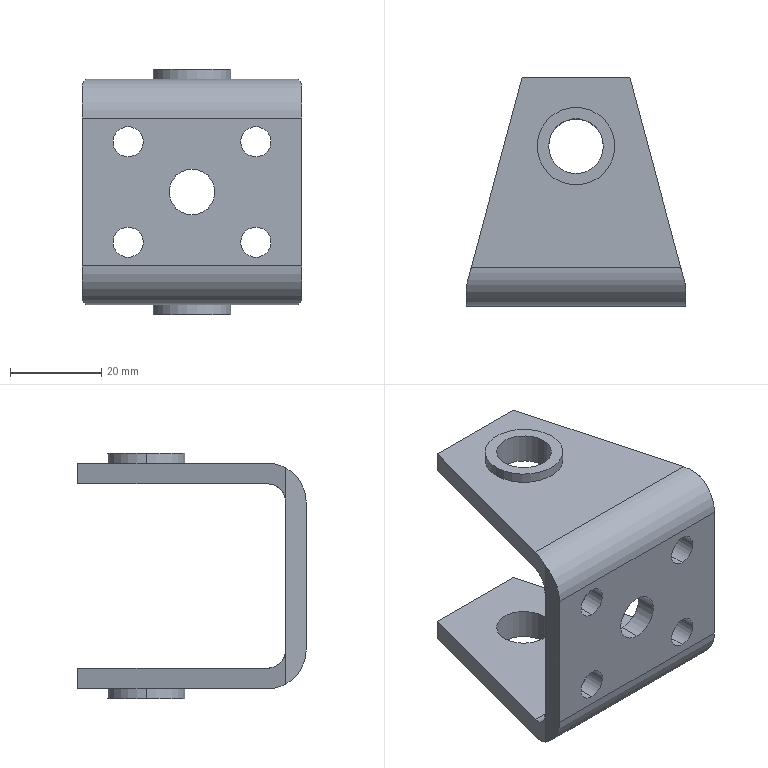Part | SolidWorks | features BaseBody 1 | 1 solid | 38 faces | box 48 x 50 x 53.8 mm | volume 22684 mm3 | cylinder 22 | plane 16 | commonest cylinder face diameters 6.6 x8 17 x6 12 x4 8 x2 10 x2
STEP:
#1=CARTESIAN_POINT('',(-8.5,0.,-24.7));
#2=VERTEX_POINT('',#1);
#3=CARTESIAN_POINT('',(8.5,0.,-24.7));
#4=VERTEX_POINT('',#3);
#5=CARTESIAN_POINT('',(0.,0.,-24.7));
#6=DIRECTION('',(0.,0.,-1.));
#7=DIRECTION('',(1.,0.,0.));
#8=AXIS2_PLACEMENT_3D('',#5,#6,#7);
#9=CIRCLE('',#8,8.5);
#10=EDGE_CURVE('',#2,#4,#9,.T.);
#11=ORIENTED_EDGE('',*,*,#10,.T.);
#12=CARTESIAN_POINT('',(8.5,0.,-26.9));
#13=VERTEX_POINT('',#12);
#14=CARTESIAN_POINT('',(8.5,0.,-26.9));
#15=DIRECTION('',(0.,0.,-1.));
#16=VECTOR('',#15,1000.);
#17=LINE('',#14,#16);
#18=EDGE_CURVE('',#4,#13,#17,.T.);
#19=ORIENTED_EDGE('',*,*,#18,.T.);
#20=CARTESIAN_POINT('',(-8.5,0.,-26.9));
#21=VERTEX_POINT('',#20);
#22=CARTESIAN_POINT('',(0.,0.,-26.9));
#23=DIRECTION('',(0.,0.,-1.));
#24=DIRECTION('',(-1.,0.,0.));
#25=AXIS2_PLACEMENT_3D('',#22,#23,#24);
#26=CIRCLE('',#25,8.5);
#27=EDGE_CURVE('',#21,#13,#26,.T.);
#28=ORIENTED_EDGE('',*,*,#27,.F.);
#29=CARTESIAN_POINT('',(-8.5,0.,-26.9));
#30=DIRECTION('',(0.,0.,-1.));
#31=VECTOR('',#30,1000.);
#32=LINE('',#29,#31);
#33=EDGE_CURVE('',#2,#21,#32,.T.);
#34=ORIENTED_EDGE('',*,*,#33,.F.);
#35=EDGE_LOOP('',(#11,#19,#28,#34));
#36=FACE_OUTER_BOUND('',#35,.T.);
#37=CARTESIAN_POINT('',(0.,0.,-26.9));
#38=DIRECTION('',(0.,0.,-1.));
#39=DIRECTION('',(-1.,0.,0.));
#40=AXIS2_PLACEMENT_3D('',#37,#38,#39);
#41=CYLINDRICAL_SURFACE('',#40,8.5);
#42=ADVANCED_FACE('',(#36),#41,.T.);
#43=CARTESIAN_POINT('',(-6.,0.,-20.2));
#44=VERTEX_POINT('',#43);
#45=CARTESIAN_POINT('',(6.,0.,-20.2));
#46=VERTEX_POINT('',#45);
#47=CARTESIAN_POINT('',(0.,0.,-20.2));
#48=DIRECTION('',(0.,0.,1.));
#49=DIRECTION('',(-1.,0.,0.));
#50=AXIS2_PLACEMENT_3D('',#47,#48,#49);
#51=CIRCLE('',#50,6.);
#52=EDGE_CURVE('',#44,#46,#51,.T.);
#53=ORIENTED_EDGE('',*,*,#52,.T.);
#54=CARTESIAN_POINT('',(6.,0.,-26.9));
#55=VERTEX_POINT('',#54);
#56=CARTESIAN_POINT('',(6.,0.,53.8));
#57=DIRECTION('',(0.,0.,-1.));
#58=VECTOR('',#57,1000.);
#59=LINE('',#56,#58);
#60=EDGE_CURVE('',#46,#55,#59,.T.);
#61=ORIENTED_EDGE('',*,*,#60,.T.);
#62=CARTESIAN_POINT('',(-6.,0.,-26.9));
#63=VERTEX_POINT('',#62);
#64=CARTESIAN_POINT('',(0.,0.,-26.9));
#65=DIRECTION('',(0.,0.,-1.));
#66=DIRECTION('',(1.,0.,0.));
#67=AXIS2_PLACEMENT_3D('',#64,#65,#66);
#68=CIRCLE('',#67,6.);
#69=EDGE_CURVE('',#55,#63,#68,.T.);
#70=ORIENTED_EDGE('',*,*,#69,.T.);
#71=CARTESIAN_POINT('',(-6.,0.,53.8));
#72=DIRECTION('',(0.,0.,-1.));
#73=VECTOR('',#72,1000.);
#74=LINE('',#71,#73);
#75=EDGE_CURVE('',#44,#63,#74,.T.);
#76=ORIENTED_EDGE('',*,*,#75,.F.);
#77=EDGE_LOOP('',(#53,#61,#70,#76));
#78=FACE_OUTER_BOUND('',#77,.T.);
#79=CARTESIAN_POINT('',(0.,0.,53.8));
#80=DIRECTION('',(0.,0.,-1.));
#81=DIRECTION('',(-1.,0.,0.));
#82=AXIS2_PLACEMENT_3D('',#79,#80,#81);
#83=CYLINDRICAL_SURFACE('',#82,6.);
#84=ADVANCED_FACE('',(#78),#83,.F.);
#85=CARTESIAN_POINT('',(0.,-35.,-5.));
#86=VERTEX_POINT('',#85);
#87=CARTESIAN_POINT('',(0.,-35.,5.));
#88=VERTEX_POINT('',#87);
#89=CARTESIAN_POINT('',(0.,-35.,0.));
#90=DIRECTION('',(0.,1.,0.));
#91=DIRECTION('',(0.,0.,1.));
#92=AXIS2_PLACEMENT_3D('',#89,#90,#91);
#93=CIRCLE('',#92,5.);
#94=EDGE_CURVE('',#86,#88,#93,.T.);
#95=ORIENTED_EDGE('',*,*,#94,.F.);
#96=CARTESIAN_POINT('',(0.,-30.5,-5.));
#97=VERTEX_POINT('',#96);
#98=CARTESIAN_POINT('',(0.,-50.,-5.));
#99=DIRECTION('',(0.,1.,0.));
#100=VECTOR('',#99,1000.);
#101=LINE('',#98,#100);
#102=EDGE_CURVE('',#86,#97,#101,.T.);
#103=ORIENTED_EDGE('',*,*,#102,.T.);
#104=CARTESIAN_POINT('',(0.,-30.5,5.));
#105=VERTEX_POINT('',#104);
#106=CARTESIAN_POINT('',(0.,-30.5,0.));
#107=DIRECTION('',(0.,-1.,0.));
#108=DIRECTION('',(0.,0.,-1.));
#109=AXIS2_PLACEMENT_3D('',#106,#107,#108);
#110=CIRCLE('',#109,5.);
#111=EDGE_CURVE('',#105,#97,#110,.T.);
#112=ORIENTED_EDGE('',*,*,#111,.F.);
#113=CARTESIAN_POINT('',(0.,-50.,5.));
#114=DIRECTION('',(0.,1.,0.));
#115=VECTOR('',#114,1000.);
#116=LINE('',#113,#115);
#117=EDGE_CURVE('',#88,#105,#116,.T.);
#118=ORIENTED_EDGE('',*,*,#117,.F.);
#119=EDGE_LOOP('',(#95,#103,#112,#118));
#120=FACE_OUTER_BOUND('',#119,.T.);
#121=CARTESIAN_POINT('',(0.,-50.,0.));
#122=DIRECTION('',(0.,1.,0.));
#123=DIRECTION('',(0.,0.,1.));
#124=AXIS2_PLACEMENT_3D('',#121,#122,#123);
#125=CYLINDRICAL_SURFACE('',#124,5.);
#126=ADVANCED_FACE('',(#120),#125,.F.);
#127=CARTESIAN_POINT('',(14.,-35.,-14.3));
#128=VERTEX_POINT('',#127);
#129=CARTESIAN_POINT('',(14.,-35.,-7.7));
#130=VERTEX_POINT('',#129);
#131=CARTESIAN_POINT('',(14.,-35.,-11.));
#132=DIRECTION('',(0.,1.,0.));
#133=DIRECTION('',(0.,0.,1.));
#134=AXIS2_PLACEMENT_3D('',#131,#132,#133);
#135=CIRCLE('',#134,3.3);
#136=EDGE_CURVE('',#128,#130,#135,.T.);
#137=ORIENTED_EDGE('',*,*,#136,.F.);
#138=CARTESIAN_POINT('',(14.,-30.5,-14.3));
#139=VERTEX_POINT('',#138);
#140=CARTESIAN_POINT('',(14.,-50.,-14.3));
#141=DIRECTION('',(0.,1.,0.));
#142=VECTOR('',#141,1000.);
#143=LINE('',#140,#142);
#144=EDGE_CURVE('',#128,#139,#143,.T.);
#145=ORIENTED_EDGE('',*,*,#144,.T.);
#146=CARTESIAN_POINT('',(14.,-30.5,-7.7));
#147=VERTEX_POINT('',#146);
#148=CARTESIAN_POINT('',(14.,-30.5,-11.));
#149=DIRECTION('',(0.,-1.,0.));
#150=DIRECTION('',(0.,0.,-1.));
#151=AXIS2_PLACEMENT_3D('',#148,#149,#150);
#152=CIRCLE('',#151,3.3);
#153=EDGE_CURVE('',#147,#139,#152,.T.);
#154=ORIENTED_EDGE('',*,*,#153,.F.);
#155=CARTESIAN_POINT('',(14.,-50.,-7.7));
#156=DIRECTION('',(0.,1.,0.));
#157=VECTOR('',#156,1000.);
#158=LINE('',#155,#157);
#159=EDGE_CURVE('',#130,#147,#158,.T.);
#160=ORIENTED_EDGE('',*,*,#159,.F.);
#161=EDGE_LOOP('',(#137,#145,#154,#160));
#162=FACE_OUTER_BOUND('',#161,.T.);
#163=CARTESIAN_POINT('',(14.,-50.,-11.));
#164=DIRECTION('',(0.,1.,0.));
#165=DIRECTION('',(0.,0.,1.));
#166=AXIS2_PLACEMENT_3D('',#163,#164,#165);
#167=CYLINDRICAL_SURFACE('',#166,3.3);
#168=ADVANCED_FACE('',(#162),#167,.F.);
#169=CARTESIAN_POINT('',(-14.,-35.,-14.3));
#170=VERTEX_POINT('',#169);
#171=CARTESIAN_POINT('',(-14.,-35.,-7.7));
#172=VERTEX_POINT('',#171);
#173=CARTESIAN_POINT('',(-14.,-35.,-11.));
#174=DIRECTION('',(0.,1.,0.));
#175=DIRECTION('',(0.,0.,1.));
#176=AXIS2_PLACEMENT_3D('',#173,#174,#175);
#177=CIRCLE('',#176,3.3);
#178=EDGE_CURVE('',#170,#172,#177,.T.);
#179=ORIENTED_EDGE('',*,*,#178,.F.);
#180=CARTESIAN_POINT('',(-14.,-30.5,-14.3));
#181=VERTEX_POINT('',#180);
#182=CARTESIAN_POINT('',(-14.,-50.,-14.3));
#183=DIRECTION('',(0.,1.,0.));
#184=VECTOR('',#183,1000.);
#185=LINE('',#182,#184);
#186=EDGE_CURVE('',#170,#181,#185,.T.);
#187=ORIENTED_EDGE('',*,*,#186,.T.);
#188=CARTESIAN_POINT('',(-14.,-30.5,-7.7));
#189=VERTEX_POINT('',#188);
#190=CARTESIAN_POINT('',(-14.,-30.5,-11.));
#191=DIRECTION('',(0.,-1.,0.));
#192=DIRECTION('',(0.,0.,-1.));
#193=AXIS2_PLACEMENT_3D('',#190,#191,#192);
#194=CIRCLE('',#193,3.3);
#195=EDGE_CURVE('',#189,#181,#194,.T.);
#196=ORIENTED_EDGE('',*,*,#195,.F.);
#197=CARTESIAN_POINT('',(-14.,-50.,-7.7));
#198=DIRECTION('',(0.,1.,0.));
#199=VECTOR('',#198,1000.);
#200=LINE('',#197,#199);
#201=EDGE_CURVE('',#172,#189,#200,.T.);
#202=ORIENTED_EDGE('',*,*,#201,.F.);
#203=EDGE_LOOP('',(#179,#187,#196,#202));
#204=FACE_OUTER_BOUND('',#203,.T.);
#205=CARTESIAN_POINT('',(-14.,-50.,-11.));
#206=DIRECTION('',(0.,1.,0.));
#207=DIRECTION('',(0.,0.,1.));
#208=AXIS2_PLACEMENT_3D('',#205,#206,#207);
#209=CYLINDRICAL_SURFACE('',#208,3.3);
#210=ADVANCED_FACE('',(#204),#209,.F.);
#211=CARTESIAN_POINT('',(-14.,-35.,7.7));
#212=VERTEX_POINT('',#211);
#213=CARTESIAN_POINT('',(-14.,-35.,14.3));
#214=VERTEX_POINT('',#213);
#215=CARTESIAN_POINT('',(-14.,-35.,11.));
#216=DIRECTION('',(0.,1.,0.));
#217=DIRECTION('',(0.,0.,1.));
#218=AXIS2_PLACEMENT_3D('',#215,#216,#217);
#219=CIRCLE('',#218,3.3);
#220=EDGE_CURVE('',#212,#214,#219,.T.);
#221=ORIENTED_EDGE('',*,*,#220,.F.);
#222=CARTESIAN_POINT('',(-14.,-30.5,7.7));
#223=VERTEX_POINT('',#222);
#224=CARTESIAN_POINT('',(-14.,-50.,7.7));
#225=DIRECTION('',(0.,1.,0.));
#226=VECTOR('',#225,1000.);
#227=LINE('',#224,#226);
#228=EDGE_CURVE('',#212,#223,#227,.T.);
#229=ORIENTED_EDGE('',*,*,#228,.T.);
#230=CARTESIAN_POINT('',(-14.,-30.5,14.3));
#231=VERTEX_POINT('',#230);
#232=CARTESIAN_POINT('',(-14.,-30.5,11.));
#233=DIRECTION('',(0.,-1.,0.));
#234=DIRECTION('',(0.,0.,-1.));
#235=AXIS2_PLACEMENT_3D('',#232,#233,#234);
#236=CIRCLE('',#235,3.3);
#237=EDGE_CURVE('',#231,#223,#236,.T.);
#238=ORIENTED_EDGE('',*,*,#237,.F.);
#239=CARTESIAN_POINT('',(-14.,-50.,14.3));
#240=DIRECTION('',(0.,1.,0.));
#241=VECTOR('',#240,1000.);
#242=LINE('',#239,#241);
#243=EDGE_CURVE('',#214,#231,#242,.T.);
#244=ORIENTED_EDGE('',*,*,#243,.F.);
#245=EDGE_LOOP('',(#221,#229,#238,#244));
#246=FACE_OUTER_BOUND('',#245,.T.);
#247=CARTESIAN_POINT('',(-14.,-50.,11.));
#248=DIRECTION('',(0.,1.,0.));
#249=DIRECTION('',(0.,0.,1.));
#250=AXIS2_PLACEMENT_3D('',#247,#248,#249);
#251=CYLINDRICAL_SURFACE('',#250,3.3);
#252=ADVANCED_FACE('',(#246),#251,.F.);
#253=CARTESIAN_POINT('',(14.,-35.,7.7));
#254=VERTEX_POINT('',#253);
#255=CARTESIAN_POINT('',(14.,-35.,14.3));
#256=VERTEX_POINT('',#255);
#257=CARTESIAN_POINT('',(14.,-35.,11.));
#258=DIRECTION('',(0.,1.,0.));
#259=DIRECTION('',(0.,0.,1.));
#260=AXIS2_PLACEMENT_3D('',#257,#258,#259);
#261=CIRCLE('',#260,3.3);
#262=EDGE_CURVE('',#254,#256,#261,.T.);
#263=ORIENTED_EDGE('',*,*,#262,.F.);
#264=CARTESIAN_POINT('',(14.,-30.5,7.7));
#265=VERTEX_POINT('',#264);
#266=CARTESIAN_POINT('',(14.,-50.,7.7));
#267=DIRECTION('',(0.,1.,0.));
#268=VECTOR('',#267,1000.);
#269=LINE('',#266,#268);
#270=EDGE_CURVE('',#254,#265,#269,.T.);
#271=ORIENTED_EDGE('',*,*,#270,.T.);
#272=CARTESIAN_POINT('',(14.,-30.5,14.3));
#273=VERTEX_POINT('',#272);
#274=CARTESIAN_POINT('',(14.,-30.5,11.));
#275=DIRECTION('',(0.,-1.,0.));
#276=DIRECTION('',(0.,0.,-1.));
#277=AXIS2_PLACEMENT_3D('',#274,#275,#276);
#278=CIRCLE('',#277,3.3);
#279=EDGE_CURVE('',#273,#265,#278,.T.);
#280=ORIENTED_EDGE('',*,*,#279,.F.);
#281=CARTESIAN_POINT('',(14.,-50.,14.3));
#282=DIRECTION('',(0.,1.,0.));
#283=VECTOR('',#282,1000.);
#284=LINE('',#281,#283);
#285=EDGE_CURVE('',#256,#273,#284,.T.);
#286=ORIENTED_EDGE('',*,*,#285,.F.);
#287=EDGE_LOOP('',(#263,#271,#280,#286));
#288=FACE_OUTER_BOUND('',#287,.T.);
#289=CARTESIAN_POINT('',(14.,-50.,11.));
#290=DIRECTION('',(0.,1.,0.));
#291=DIRECTION('',(0.,0.,1.));
#292=AXIS2_PLACEMENT_3D('',#289,#290,#291);
#293=CYLINDRICAL_SURFACE('',#292,3.3);
#294=ADVANCED_FACE('',(#288),#293,.F.);
#295=CARTESIAN_POINT('',(-8.5,0.,26.9));
#296=VERTEX_POINT('',#295);
#297=CARTESIAN_POINT('',(8.5,0.,26.9));
#298=VERTEX_POINT('',#297);
#299=CARTESIAN_POINT('',(0.,0.,26.9));
#300=DIRECTION('',(0.,0.,-1.));
#301=DIRECTION('',(-1.,0.,0.));
#302=AXIS2_PLACEMENT_3D('',#299,#300,#301);
#303=CIRCLE('',#302,8.5);
#304=EDGE_CURVE('',#296,#298,#303,.T.);
#305=ORIENTED_EDGE('',*,*,#304,.T.);
#306=CARTESIAN_POINT('',(8.5,0.,24.7));
#307=VERTEX_POINT('',#306);
#308=CARTESIAN_POINT('',(8.5,0.,-26.9));
#309=DIRECTION('',(0.,0.,-1.));
#310=VECTOR('',#309,1000.);
#311=LINE('',#308,#310);
#312=EDGE_CURVE('',#298,#307,#311,.T.);
#313=ORIENTED_EDGE('',*,*,#312,.T.);
#314=CARTESIAN_POINT('',(-8.5,0.,24.7));
#315=VERTEX_POINT('',#314);
#316=CARTESIAN_POINT('',(0.,0.,24.7));
#317=DIRECTION('',(0.,0.,1.));
#318=DIRECTION('',(-1.,0.,0.));
#319=AXIS2_PLACEMENT_3D('',#316,#317,#318);
#320=CIRCLE('',#319,8.5);
#321=EDGE_CURVE('',#307,#315,#320,.T.);
#322=ORIENTED_EDGE('',*,*,#321,.T.);
#323=CARTESIAN_POINT('',(-8.5,0.,-26.9));
#324=DIRECTION('',(0.,0.,-1.));
#325=VECTOR('',#324,1000.);
#326=LINE('',#323,#325);
#327=EDGE_CURVE('',#296,#315,#326,.T.);
#328=ORIENTED_EDGE('',*,*,#327,.F.);
#329=EDGE_LOOP('',(#305,#313,#322,#328));
#330=FACE_OUTER_BOUND('',#329,.T.);
#331=CARTESIAN_POINT('',(0.,0.,-26.9));
#332=DIRECTION('',(0.,0.,-1.));
#333=DIRECTION('',(-1.,0.,0.));
#334=AXIS2_PLACEMENT_3D('',#331,#332,#333);
#335=CYLINDRICAL_SURFACE('',#334,8.5);
#336=ADVANCED_FACE('',(#330),#335,.T.);
#337=CARTESIAN_POINT('',(-6.,0.,26.9));
#338=VERTEX_POINT('',#337);
#339=CARTESIAN_POINT('',(6.,0.,26.9));
#340=VERTEX_POINT('',#339);
#341=CARTESIAN_POINT('',(0.,0.,26.9));
#342=DIRECTION('',(0.,0.,1.));
#343=DIRECTION('',(-1.,0.,0.));
#344=AXIS2_PLACEMENT_3D('',#341,#342,#343);
#345=CIRCLE('',#344,6.);
#346=EDGE_CURVE('',#338,#340,#345,.T.);
#347=ORIENTED_EDGE('',*,*,#346,.T.);
#348=CARTESIAN_POINT('',(6.,0.,20.2));
#349=VERTEX_POINT('',#348);
#350=CARTESIAN_POINT('',(6.,0.,53.8));
#351=DIRECTION('',(0.,0.,-1.));
#352=VECTOR('',#351,1000.);
#353=LINE('',#350,#352);
#354=EDGE_CURVE('',#340,#349,#353,.T.);
#355=ORIENTED_EDGE('',*,*,#354,.T.);
#356=CARTESIAN_POINT('',(-6.,0.,20.2));
#357=VERTEX_POINT('',#356);
#358=CARTESIAN_POINT('',(0.,0.,20.2));
#359=DIRECTION('',(0.,0.,-1.));
#360=DIRECTION('',(1.,0.,0.));
#361=AXIS2_PLACEMENT_3D('',#358,#359,#360);
#362=CIRCLE('',#361,6.);
#363=EDGE_CURVE('',#349,#357,#362,.T.);
#364=ORIENTED_EDGE('',*,*,#363,.T.);
#365=CARTESIAN_POINT('',(-6.,0.,53.8));
#366=DIRECTION('',(0.,0.,-1.));
#367=VECTOR('',#366,1000.);
#368=LINE('',#365,#367);
#369=EDGE_CURVE('',#338,#357,#368,.T.);
#370=ORIENTED_EDGE('',*,*,#369,.F.);
#371=EDGE_LOOP('',(#347,#355,#364,#370));
#372=FACE_OUTER_BOUND('',#371,.T.);
#373=CARTESIAN_POINT('',(0.,0.,53.8));
#374=DIRECTION('',(0.,0.,-1.));
#375=DIRECTION('',(-1.,0.,0.));
#376=AXIS2_PLACEMENT_3D('',#373,#374,#375);
#377=CYLINDRICAL_SURFACE('',#376,6.);
#378=ADVANCED_FACE('',(#372),#377,.F.);
#379=CARTESIAN_POINT('',(11.8,15.,20.2));
#380=VERTEX_POINT('',#379);
#381=CARTESIAN_POINT('',(-11.8,15.,20.2));
#382=VERTEX_POINT('',#381);
#383=CARTESIAN_POINT('',(11.8,15.,20.2));
#384=DIRECTION('',(-1.,0.,0.));
#385=VECTOR('',#384,1000.);
#386=LINE('',#383,#385);
#387=EDGE_CURVE('',#380,#382,#386,.T.);
#388=ORIENTED_EDGE('',*,*,#387,.T.);
#389=CARTESIAN_POINT('',(-11.8,15.,24.7));
#390=VERTEX_POINT('',#389);
#391=CARTESIAN_POINT('',(-11.8,15.,24.7));
#392=DIRECTION('',(0.,0.,-1.));
#393=VECTOR('',#392,1000.);
#394=LINE('',#391,#393);
#395=EDGE_CURVE('',#390,#382,#394,.T.);
#396=ORIENTED_EDGE('',*,*,#395,.F.);
#397=CARTESIAN_POINT('',(11.8,15.,24.7));
#398=VERTEX_POINT('',#397);
#399=CARTESIAN_POINT('',(11.8,15.,24.7));
#400=DIRECTION('',(-1.,0.,0.));
#401=VECTOR('',#400,1000.);
#402=LINE('',#399,#401);
#403=EDGE_CURVE('',#398,#390,#402,.T.);
#404=ORIENTED_EDGE('',*,*,#403,.F.);
#405=CARTESIAN_POINT('',(11.8,15.,24.7));
#406=DIRECTION('',(0.,0.,-1.));
#407=VECTOR('',#406,1000.);
#408=LINE('',#405,#407);
#409=EDGE_CURVE('',#398,#380,#408,.T.);
#410=ORIENTED_EDGE('',*,*,#409,.T.);
#411=EDGE_LOOP('',(#388,#396,#404,#410));
#412=FACE_OUTER_BOUND('',#411,.T.);
#413=CARTESIAN_POINT('',(24.,15.,20.2));
#414=DIRECTION('',(0.,-1.,0.));
#415=DIRECTION('',(0.,0.,-1.));
#416=AXIS2_PLACEMENT_3D('',#413,#414,#415);
#417=PLANE('',#416);
#418=ADVANCED_FACE('',(#412),#417,.F.);
#419=CARTESIAN_POINT('',(0.,0.,20.2));
#420=DIRECTION('',(0.,0.,-1.));
#421=DIRECTION('',(1.,0.,0.));
#422=AXIS2_PLACEMENT_3D('',#419,#420,#421);
#423=CIRCLE('',#422,6.);
#424=EDGE_CURVE('',#357,#349,#423,.T.);
#425=ORIENTED_EDGE('',*,*,#424,.F.);
#426=ORIENTED_EDGE('',*,*,#363,.F.);
#427=EDGE_LOOP('',(#425,#426));
#428=FACE_BOUND('',#427,.T.);
#429=CARTESIAN_POINT('',(22.927,-26.5,20.2));
#430=VERTEX_POINT('',#429);
#431=CARTESIAN_POINT('',(-22.927,-26.5,20.2));
#432=VERTEX_POINT('',#431);
#433=CARTESIAN_POINT('',(22.927,-26.5,20.2));
#434=DIRECTION('',(-1.,0.,0.));
#435=VECTOR('',#434,1000.);
#436=LINE('',#433,#435);
#437=EDGE_CURVE('',#430,#432,#436,.T.);
#438=ORIENTED_EDGE('',*,*,#437,.T.);
#439=CARTESIAN_POINT('',(-22.927,-26.5,20.2));
#440=DIRECTION('',(0.259,0.9659,0.));
#441=VECTOR('',#440,1000.);
#442=LINE('',#439,#441);
#443=EDGE_CURVE('',#432,#382,#442,.T.);
#444=ORIENTED_EDGE('',*,*,#443,.T.);
#445=ORIENTED_EDGE('',*,*,#387,.F.);
#446=CARTESIAN_POINT('',(11.8,15.,20.2));
#447=DIRECTION('',(0.259,-0.9659,0.));
#448=VECTOR('',#447,1000.);
#449=LINE('',#446,#448);
#450=EDGE_CURVE('',#380,#430,#449,.T.);
#451=ORIENTED_EDGE('',*,*,#450,.T.);
#452=EDGE_LOOP('',(#438,#444,#445,#451));
#453=FACE_OUTER_BOUND('',#452,.T.);
#454=CARTESIAN_POINT('',(24.,-26.5,20.2));
#455=DIRECTION('',(0.,0.,1.));
#456=DIRECTION('',(1.,0.,0.));
#457=AXIS2_PLACEMENT_3D('',#454,#455,#456);
#458=PLANE('',#457);
#459=ADVANCED_FACE('',(#428,#453),#458,.F.);
#460=ORIENTED_EDGE('',*,*,#395,.T.);
#461=ORIENTED_EDGE('',*,*,#443,.F.);
#462=CARTESIAN_POINT('',(-24.,-30.5,16.2));
#463=VERTEX_POINT('',#462);
#464=CARTESIAN_POINT('',(-22.927,-26.5,20.2));
#465=CARTESIAN_POINT('',(-23.069,-27.029,20.2));
#466=CARTESIAN_POINT('',(-23.207,-27.542,20.098));
#467=CARTESIAN_POINT('',(-23.469,-28.519,19.693));
#468=CARTESIAN_POINT('',(-23.585,-28.954,19.403));
#469=CARTESIAN_POINT('',(-23.736,-29.515,18.842));
#470=CARTESIAN_POINT('',(-23.781,-29.682,18.639));
#471=CARTESIAN_POINT('',(-23.858,-29.971,18.206));
#472=CARTESIAN_POINT('',(-23.891,-30.094,17.976));
#473=CARTESIAN_POINT('',(-23.973,-30.398,17.241));
#474=CARTESIAN_POINT('',(-24.,-30.5,16.732));
#475=CARTESIAN_POINT('',(-24.,-30.5,16.2));
#476=B_SPLINE_CURVE_WITH_KNOTS('',3,(#464,#465,#466,#467,#468,#469,#470,#471,#472,#473,#474,#475),.UNSPECIFIED.,.F.,.F.,(4,2,2,2,2,4),(4.712,5.105,5.498,5.694,5.89,6.283),.UNSPECIFIED.);
#477=EDGE_CURVE('',#432,#463,#476,.T.);
#478=ORIENTED_EDGE('',*,*,#477,.T.);
#479=CARTESIAN_POINT('',(-24.,-30.5,23.7));
#480=VERTEX_POINT('',#479);
#481=CARTESIAN_POINT('',(-24.,-30.5,23.7));
#482=DIRECTION('',(0.,0.,-1.));
#483=VECTOR('',#482,1000.);
#484=LINE('',#481,#483);
#485=EDGE_CURVE('',#480,#463,#484,.T.);
#486=ORIENTED_EDGE('',*,*,#485,.F.);
#487=CARTESIAN_POINT('',(-22.927,-26.5,24.7));
#488=VERTEX_POINT('',#487);
#489=CARTESIAN_POINT('',(-22.927,-26.5,24.7));
#490=CARTESIAN_POINT('',(-23.113,-27.194,24.7));
#491=CARTESIAN_POINT('',(-23.3,-27.889,24.614));
#492=CARTESIAN_POINT('',(-23.661,-29.235,24.278));
#493=CARTESIAN_POINT('',(-23.835,-29.886,24.028));
#494=CARTESIAN_POINT('',(-24.,-30.5,23.7));
#495=B_SPLINE_CURVE_WITH_KNOTS('',3,(#489,#490,#491,#492,#493,#494),.UNSPECIFIED.,.F.,.F.,(4,2,4),(4.712,4.957,5.202),.UNSPECIFIED.);
#496=EDGE_CURVE('',#488,#480,#495,.T.);
#497=ORIENTED_EDGE('',*,*,#496,.F.);
#498=CARTESIAN_POINT('',(-11.8,15.,24.7));
#499=DIRECTION('',(-0.259,-0.9659,0.));
#500=VECTOR('',#499,1000.);
#501=LINE('',#498,#500);
#502=EDGE_CURVE('',#390,#488,#501,.T.);
#503=ORIENTED_EDGE('',*,*,#502,.F.);
#504=EDGE_LOOP('',(#460,#461,#478,#486,#497,#503));
#505=FACE_OUTER_BOUND('',#504,.T.);
#506=CARTESIAN_POINT('',(-11.8,15.,53.8));
#507=DIRECTION('',(0.9659,-0.259,0.));
#508=DIRECTION('',(0.259,0.9659,0.));
#509=AXIS2_PLACEMENT_3D('',#506,#507,#508);
#510=PLANE('',#509);
#511=ADVANCED_FACE('',(#505),#510,.F.);
#512=CARTESIAN_POINT('',(0.,0.,24.7));
#513=DIRECTION('',(0.,0.,1.));
#514=DIRECTION('',(-1.,0.,0.));
#515=AXIS2_PLACEMENT_3D('',#512,#513,#514);
#516=CIRCLE('',#515,8.5);
#517=EDGE_CURVE('',#315,#307,#516,.T.);
#518=ORIENTED_EDGE('',*,*,#517,.F.);
#519=ORIENTED_EDGE('',*,*,#321,.F.);
#520=EDGE_LOOP('',(#518,#519));
#521=FACE_BOUND('',#520,.T.);
#522=ORIENTED_EDGE('',*,*,#403,.T.);
#523=ORIENTED_EDGE('',*,*,#502,.T.);
#524=CARTESIAN_POINT('',(22.927,-26.5,24.7));
#525=VERTEX_POINT('',#524);
#526=CARTESIAN_POINT('',(22.927,-26.5,24.7));
#527=DIRECTION('',(-1.,0.,0.));
#528=VECTOR('',#527,1000.);
#529=LINE('',#526,#528);
#530=EDGE_CURVE('',#525,#488,#529,.T.);
#531=ORIENTED_EDGE('',*,*,#530,.F.);
#532=CARTESIAN_POINT('',(22.927,-26.5,24.7));
#533=DIRECTION('',(-0.259,0.9659,0.));
#534=VECTOR('',#533,1000.);
#535=LINE('',#532,#534);
#536=EDGE_CURVE('',#525,#398,#535,.T.);
#537=ORIENTED_EDGE('',*,*,#536,.T.);
#538=EDGE_LOOP('',(#522,#523,#531,#537));
#539=FACE_OUTER_BOUND('',#538,.T.);
#540=CARTESIAN_POINT('',(24.,15.,24.7));
#541=DIRECTION('',(0.,0.,-1.));
#542=DIRECTION('',(-1.,0.,0.));
#543=AXIS2_PLACEMENT_3D('',#540,#541,#542);
#544=PLANE('',#543);
#545=ADVANCED_FACE('',(#521,#539),#544,.F.);
#546=CARTESIAN_POINT('',(24.,-30.5,23.7));
#547=VERTEX_POINT('',#546);
#548=CARTESIAN_POINT('',(24.,-30.5,23.7));
#549=CARTESIAN_POINT('',(23.835,-29.886,24.028));
#550=CARTESIAN_POINT('',(23.661,-29.235,24.278));
#551=CARTESIAN_POINT('',(23.3,-27.889,24.614));
#552=CARTESIAN_POINT('',(23.113,-27.194,24.7));
#553=CARTESIAN_POINT('',(22.927,-26.5,24.7));
#554=B_SPLINE_CURVE_WITH_KNOTS('',3,(#548,#549,#550,#551,#552,#553),.UNSPECIFIED.,.F.,.F.,(4,2,4),(4.222,4.467,4.712),.UNSPECIFIED.);
#555=EDGE_CURVE('',#547,#525,#554,.T.);
#556=ORIENTED_EDGE('',*,*,#555,.F.);
#557=CARTESIAN_POINT('',(24.,-30.5,16.2));
#558=VERTEX_POINT('',#557);
#559=CARTESIAN_POINT('',(24.,-30.5,23.7));
#560=DIRECTION('',(0.,0.,-1.));
#561=VECTOR('',#560,1000.);
#562=LINE('',#559,#561);
#563=EDGE_CURVE('',#547,#558,#562,.T.);
#564=ORIENTED_EDGE('',*,*,#563,.T.);
#565=CARTESIAN_POINT('',(24.,-30.5,16.2));
#566=CARTESIAN_POINT('',(24.,-30.5,16.732));
#567=CARTESIAN_POINT('',(23.973,-30.398,17.241));
#568=CARTESIAN_POINT('',(23.891,-30.094,17.976));
#569=CARTESIAN_POINT('',(23.858,-29.971,18.206));
#570=CARTESIAN_POINT('',(23.781,-29.682,18.639));
#571=CARTESIAN_POINT('',(23.736,-29.515,18.842));
#572=CARTESIAN_POINT('',(23.585,-28.954,19.403));
#573=CARTESIAN_POINT('',(23.469,-28.519,19.693));
#574=CARTESIAN_POINT('',(23.207,-27.542,20.098));
#575=CARTESIAN_POINT('',(23.069,-27.029,20.2));
#576=CARTESIAN_POINT('',(22.927,-26.5,20.2));
#577=B_SPLINE_CURVE_WITH_KNOTS('',3,(#565,#566,#567,#568,#569,#570,#571,#572,#573,#574,#575,#576),.UNSPECIFIED.,.F.,.F.,(4,2,2,2,2,4),(3.142,3.534,3.731,3.927,4.32,4.712),.UNSPECIFIED.);
#578=EDGE_CURVE('',#558,#430,#577,.T.);
#579=ORIENTED_EDGE('',*,*,#578,.T.);
#580=ORIENTED_EDGE('',*,*,#450,.F.);
#581=ORIENTED_EDGE('',*,*,#409,.F.);
#582=ORIENTED_EDGE('',*,*,#536,.F.);
#583=EDGE_LOOP('',(#556,#564,#579,#580,#581,#582));
#584=FACE_OUTER_BOUND('',#583,.T.);
#585=CARTESIAN_POINT('',(24.,-30.5,53.8));
#586=DIRECTION('',(-0.9659,-0.259,0.));
#587=DIRECTION('',(0.259,-0.9659,0.));
#588=AXIS2_PLACEMENT_3D('',#585,#586,#587);
#589=PLANE('',#588);
#590=ADVANCED_FACE('',(#584),#589,.F.);
#591=ORIENTED_EDGE('',*,*,#354,.F.);
#592=CARTESIAN_POINT('',(0.,0.,26.9));
#593=DIRECTION('',(0.,0.,1.));
#594=DIRECTION('',(-1.,0.,0.));
#595=AXIS2_PLACEMENT_3D('',#592,#593,#594);
#596=CIRCLE('',#595,6.);
#597=EDGE_CURVE('',#340,#338,#596,.T.);
#598=ORIENTED_EDGE('',*,*,#597,.T.);
#599=ORIENTED_EDGE('',*,*,#369,.T.);
#600=ORIENTED_EDGE('',*,*,#424,.T.);
#601=EDGE_LOOP('',(#591,#598,#599,#600));
#602=FACE_OUTER_BOUND('',#601,.T.);
#603=CARTESIAN_POINT('',(0.,0.,53.8));
#604=DIRECTION('',(0.,0.,-1.));
#605=DIRECTION('',(-1.,0.,0.));
#606=AXIS2_PLACEMENT_3D('',#603,#604,#605);
#607=CYLINDRICAL_SURFACE('',#606,6.);
#608=ADVANCED_FACE('',(#602),#607,.F.);
#609=ORIENTED_EDGE('',*,*,#477,.F.);
#610=ORIENTED_EDGE('',*,*,#437,.F.);
#611=ORIENTED_EDGE('',*,*,#578,.F.);
#612=CARTESIAN_POINT('',(24.,-30.5,16.2));
#613=DIRECTION('',(-1.,0.,0.));
#614=VECTOR('',#613,1000.);
#615=LINE('',#612,#614);
#616=EDGE_CURVE('',#558,#463,#615,.T.);
#617=ORIENTED_EDGE('',*,*,#616,.T.);
#618=EDGE_LOOP('',(#609,#610,#611,#617));
#619=FACE_OUTER_BOUND('',#618,.T.);
#620=CARTESIAN_POINT('',(24.,-26.5,16.2));
#621=DIRECTION('',(-1.,0.,0.));
#622=DIRECTION('',(0.,0.,1.));
#623=AXIS2_PLACEMENT_3D('',#620,#621,#622);
#624=CYLINDRICAL_SURFACE('',#623,4.);
#625=ADVANCED_FACE('',(#619),#624,.F.);
#626=CARTESIAN_POINT('',(-24.,-35.,16.2));
#627=VERTEX_POINT('',#626);
#628=CARTESIAN_POINT('',(-24.,-26.5,16.2));
#629=DIRECTION('',(1.,0.,0.));
#630=DIRECTION('',(0.,-0.4706,0.8824));
#631=AXIS2_PLACEMENT_3D('',#628,#629,#630);
#632=CIRCLE('',#631,8.5);
#633=EDGE_CURVE('',#480,#627,#632,.T.);
#634=ORIENTED_EDGE('',*,*,#633,.F.);
#635=ORIENTED_EDGE('',*,*,#485,.T.);
#636=CARTESIAN_POINT('',(-24.,-30.5,-16.2));
#637=VERTEX_POINT('',#636);
#638=CARTESIAN_POINT('',(-24.,-30.5,-16.2));
#639=DIRECTION('',(0.,0.,1.));
#640=VECTOR('',#639,1000.);
#641=LINE('',#638,#640);
#642=EDGE_CURVE('',#637,#463,#641,.T.);
#643=ORIENTED_EDGE('',*,*,#642,.F.);
#644=CARTESIAN_POINT('',(-24.,-30.5,-23.7));
#645=VERTEX_POINT('',#644);
#646=CARTESIAN_POINT('',(-24.,-30.5,-16.2));
#647=DIRECTION('',(0.,0.,-1.));
#648=VECTOR('',#647,1000.);
#649=LINE('',#646,#648);
#650=EDGE_CURVE('',#637,#645,#649,.T.);
#651=ORIENTED_EDGE('',*,*,#650,.T.);
#652=CARTESIAN_POINT('',(-24.,-35.,-16.2));
#653=VERTEX_POINT('',#652);
#654=CARTESIAN_POINT('',(-24.,-26.5,-16.2));
#655=DIRECTION('',(1.,0.,0.));
#656=DIRECTION('',(0.,-1.,0.));
#657=AXIS2_PLACEMENT_3D('',#654,#655,#656);
#658=CIRCLE('',#657,8.5);
#659=EDGE_CURVE('',#653,#645,#658,.T.);
#660=ORIENTED_EDGE('',*,*,#659,.F.);
#661=CARTESIAN_POINT('',(-24.,-35.,16.2));
#662=DIRECTION('',(0.,0.,-1.));
#663=VECTOR('',#662,1000.);
#664=LINE('',#661,#663);
#665=EDGE_CURVE('',#627,#653,#664,.T.);
#666=ORIENTED_EDGE('',*,*,#665,.F.);
#667=EDGE_LOOP('',(#634,#635,#643,#651,#660,#666));
#668=FACE_OUTER_BOUND('',#667,.T.);
#669=CARTESIAN_POINT('',(-24.,-26.5,16.2));
#670=DIRECTION('',(1.,0.,0.));
#671=DIRECTION('',(0.,0.,-1.));
#672=AXIS2_PLACEMENT_3D('',#669,#670,#671);
#673=PLANE('',#672);
#674=ADVANCED_FACE('',(#668),#673,.F.);
#675=ORIENTED_EDGE('',*,*,#530,.T.);
#676=ORIENTED_EDGE('',*,*,#496,.T.);
#677=ORIENTED_EDGE('',*,*,#633,.T.);
#678=CARTESIAN_POINT('',(24.,-35.,16.2));
#679=VERTEX_POINT('',#678);
#680=CARTESIAN_POINT('',(24.,-35.,16.2));
#681=DIRECTION('',(-1.,0.,0.));
#682=VECTOR('',#681,1000.);
#683=LINE('',#680,#682);
#684=EDGE_CURVE('',#679,#627,#683,.T.);
#685=ORIENTED_EDGE('',*,*,#684,.F.);
#686=CARTESIAN_POINT('',(24.,-26.5,16.2));
#687=DIRECTION('',(1.,0.,0.));
#688=DIRECTION('',(0.,-0.4706,0.8824));
#689=AXIS2_PLACEMENT_3D('',#686,#687,#688);
#690=CIRCLE('',#689,8.5);
#691=EDGE_CURVE('',#547,#679,#690,.T.);
#692=ORIENTED_EDGE('',*,*,#691,.F.);
#693=ORIENTED_EDGE('',*,*,#555,.T.);
#694=EDGE_LOOP('',(#675,#676,#677,#685,#692,#693));
#695=FACE_OUTER_BOUND('',#694,.T.);
#696=CARTESIAN_POINT('',(24.,-26.5,16.2));
#697=DIRECTION('',(-1.,0.,0.));
#698=DIRECTION('',(0.,0.,1.));
#699=AXIS2_PLACEMENT_3D('',#696,#697,#698);
#700=CYLINDRICAL_SURFACE('',#699,8.5);
#701=ADVANCED_FACE('',(#695),#700,.T.);
#702=ORIENTED_EDGE('',*,*,#312,.F.);
#703=CARTESIAN_POINT('',(0.,0.,26.9));
#704=DIRECTION('',(0.,0.,-1.));
#705=DIRECTION('',(-1.,0.,0.));
#706=AXIS2_PLACEMENT_3D('',#703,#704,#705);
#707=CIRCLE('',#706,8.5);
#708=EDGE_CURVE('',#298,#296,#707,.T.);
#709=ORIENTED_EDGE('',*,*,#708,.T.);
#710=ORIENTED_EDGE('',*,*,#327,.T.);
#711=ORIENTED_EDGE('',*,*,#517,.T.);
#712=EDGE_LOOP('',(#702,#709,#710,#711));
#713=FACE_OUTER_BOUND('',#712,.T.);
#714=CARTESIAN_POINT('',(0.,0.,-26.9));
#715=DIRECTION('',(0.,0.,-1.));
#716=DIRECTION('',(-1.,0.,0.));
#717=AXIS2_PLACEMENT_3D('',#714,#715,#716);
#718=CYLINDRICAL_SURFACE('',#717,8.5);
#719=ADVANCED_FACE('',(#713),#718,.T.);
#720=ORIENTED_EDGE('',*,*,#563,.F.);
#721=ORIENTED_EDGE('',*,*,#691,.T.);
#722=CARTESIAN_POINT('',(24.,-35.,-16.2));
#723=VERTEX_POINT('',#722);
#724=CARTESIAN_POINT('',(24.,-35.,16.2));
#725=DIRECTION('',(0.,0.,-1.));
#726=VECTOR('',#725,1000.);
#727=LINE('',#724,#726);
#728=EDGE_CURVE('',#679,#723,#727,.T.);
#729=ORIENTED_EDGE('',*,*,#728,.T.);
#730=CARTESIAN_POINT('',(24.,-30.5,-23.7));
#731=VERTEX_POINT('',#730);
#732=CARTESIAN_POINT('',(24.,-26.5,-16.2));
#733=DIRECTION('',(1.,0.,0.));
#734=DIRECTION('',(0.,-1.,0.));
#735=AXIS2_PLACEMENT_3D('',#732,#733,#734);
#736=CIRCLE('',#735,8.5);
#737=EDGE_CURVE('',#723,#731,#736,.T.);
#738=ORIENTED_EDGE('',*,*,#737,.T.);
#739=CARTESIAN_POINT('',(24.,-30.5,-16.2));
#740=VERTEX_POINT('',#739);
#741=CARTESIAN_POINT('',(24.,-30.5,-16.2));
#742=DIRECTION('',(0.,0.,-1.));
#743=VECTOR('',#742,1000.);
#744=LINE('',#741,#743);
#745=EDGE_CURVE('',#740,#731,#744,.T.);
#746=ORIENTED_EDGE('',*,*,#745,.F.);
#747=CARTESIAN_POINT('',(24.,-30.5,-16.2));
#748=DIRECTION('',(0.,0.,1.));
#749=VECTOR('',#748,1000.);
#750=LINE('',#747,#749);
#751=EDGE_CURVE('',#740,#558,#750,.T.);
#752=ORIENTED_EDGE('',*,*,#751,.T.);
#753=EDGE_LOOP('',(#720,#721,#729,#738,#746,#752));
#754=FACE_OUTER_BOUND('',#753,.T.);
#755=CARTESIAN_POINT('',(24.,-26.5,16.2));
#756=DIRECTION('',(1.,0.,0.));
#757=DIRECTION('',(0.,0.,-1.));
#758=AXIS2_PLACEMENT_3D('',#755,#756,#757);
#759=PLANE('',#758);
#760=ADVANCED_FACE('',(#754),#759,.T.);
#761=ORIENTED_EDGE('',*,*,#304,.F.);
#762=ORIENTED_EDGE('',*,*,#708,.F.);
#763=EDGE_LOOP('',(#761,#762));
#764=FACE_OUTER_BOUND('',#763,.T.);
#765=ORIENTED_EDGE('',*,*,#346,.F.);
#766=ORIENTED_EDGE('',*,*,#597,.F.);
#767=EDGE_LOOP('',(#765,#766));
#768=FACE_BOUND('',#767,.T.);
#769=CARTESIAN_POINT('',(0.,0.,26.9));
#770=DIRECTION('',(0.,0.,-1.));
#771=DIRECTION('',(-1.,0.,0.));
#772=AXIS2_PLACEMENT_3D('',#769,#770,#771);
#773=PLANE('',#772);
#774=ADVANCED_FACE('',(#764,#768),#773,.F.);
#775=ORIENTED_EDGE('',*,*,#279,.T.);
#776=CARTESIAN_POINT('',(14.,-30.5,11.));
#777=DIRECTION('',(0.,-1.,0.));
#778=DIRECTION('',(0.,0.,-1.));
#779=AXIS2_PLACEMENT_3D('',#776,#777,#778);
#780=CIRCLE('',#779,3.3);
#781=EDGE_CURVE('',#265,#273,#780,.T.);
#782=ORIENTED_EDGE('',*,*,#781,.T.);
#783=EDGE_LOOP('',(#775,#782));
#784=FACE_BOUND('',#783,.T.);
#785=ORIENTED_EDGE('',*,*,#237,.T.);
#786=CARTESIAN_POINT('',(-14.,-30.5,11.));
#787=DIRECTION('',(0.,-1.,0.));
#788=DIRECTION('',(0.,0.,-1.));
#789=AXIS2_PLACEMENT_3D('',#786,#787,#788);
#790=CIRCLE('',#789,3.3);
#791=EDGE_CURVE('',#223,#231,#790,.T.);
#792=ORIENTED_EDGE('',*,*,#791,.T.);
#793=EDGE_LOOP('',(#785,#792));
#794=FACE_BOUND('',#793,.T.);
#795=ORIENTED_EDGE('',*,*,#195,.T.);
#796=CARTESIAN_POINT('',(-14.,-30.5,-11.));
#797=DIRECTION('',(0.,-1.,0.));
#798=DIRECTION('',(0.,0.,-1.));
#799=AXIS2_PLACEMENT_3D('',#796,#797,#798);
#800=CIRCLE('',#799,3.3);
#801=EDGE_CURVE('',#181,#189,#800,.T.);
#802=ORIENTED_EDGE('',*,*,#801,.T.);
#803=EDGE_LOOP('',(#795,#802));
#804=FACE_BOUND('',#803,.T.);
#805=ORIENTED_EDGE('',*,*,#153,.T.);
#806=CARTESIAN_POINT('',(14.,-30.5,-11.));
#807=DIRECTION('',(0.,-1.,0.));
#808=DIRECTION('',(0.,0.,-1.));
#809=AXIS2_PLACEMENT_3D('',#806,#807,#808);
#810=CIRCLE('',#809,3.3);
#811=EDGE_CURVE('',#139,#147,#810,.T.);
#812=ORIENTED_EDGE('',*,*,#811,.T.);
#813=EDGE_LOOP('',(#805,#812));
#814=FACE_BOUND('',#813,.T.);
#815=ORIENTED_EDGE('',*,*,#111,.T.);
#816=CARTESIAN_POINT('',(0.,-30.5,0.));
#817=DIRECTION('',(0.,-1.,0.));
#818=DIRECTION('',(0.,0.,-1.));
#819=AXIS2_PLACEMENT_3D('',#816,#817,#818);
#820=CIRCLE('',#819,5.);
#821=EDGE_CURVE('',#97,#105,#820,.T.);
#822=ORIENTED_EDGE('',*,*,#821,.T.);
#823=EDGE_LOOP('',(#815,#822));
#824=FACE_BOUND('',#823,.T.);
#825=ORIENTED_EDGE('',*,*,#642,.T.);
#826=ORIENTED_EDGE('',*,*,#616,.F.);
#827=ORIENTED_EDGE('',*,*,#751,.F.);
#828=CARTESIAN_POINT('',(24.,-30.5,-16.2));
#829=DIRECTION('',(-1.,0.,0.));
#830=VECTOR('',#829,1000.);
#831=LINE('',#828,#830);
#832=EDGE_CURVE('',#740,#637,#831,.T.);
#833=ORIENTED_EDGE('',*,*,#832,.T.);
#834=EDGE_LOOP('',(#825,#826,#827,#833));
#835=FACE_OUTER_BOUND('',#834,.T.);
#836=CARTESIAN_POINT('',(24.,-30.5,-16.2));
#837=DIRECTION('',(0.,-1.,0.));
#838=DIRECTION('',(0.,0.,-1.));
#839=AXIS2_PLACEMENT_3D('',#836,#837,#838);
#840=PLANE('',#839);
#841=ADVANCED_FACE('',(#784,#794,#804,#814,#824,#835),#840,.F.);
#842=ORIENTED_EDGE('',*,*,#650,.F.);
#843=CARTESIAN_POINT('',(-22.927,-26.5,-20.2));
#844=VERTEX_POINT('',#843);
#845=CARTESIAN_POINT('',(-24.,-30.5,-16.2));
#846=CARTESIAN_POINT('',(-24.,-30.5,-16.732));
#847=CARTESIAN_POINT('',(-23.973,-30.398,-17.241));
#848=CARTESIAN_POINT('',(-23.891,-30.094,-17.976));
#849=CARTESIAN_POINT('',(-23.858,-29.971,-18.206));
#850=CARTESIAN_POINT('',(-23.781,-29.682,-18.639));
#851=CARTESIAN_POINT('',(-23.736,-29.515,-18.842));
#852=CARTESIAN_POINT('',(-23.585,-28.954,-19.403));
#853=CARTESIAN_POINT('',(-23.469,-28.519,-19.693));
#854=CARTESIAN_POINT('',(-23.207,-27.542,-20.098));
#855=CARTESIAN_POINT('',(-23.069,-27.029,-20.2));
#856=CARTESIAN_POINT('',(-22.927,-26.5,-20.2));
#857=B_SPLINE_CURVE_WITH_KNOTS('',3,(#845,#846,#847,#848,#849,#850,#851,#852,#853,#854,#855,#856),.UNSPECIFIED.,.F.,.F.,(4,2,2,2,2,4),(0.,0.3927,0.589,0.7854,1.178,1.571),.UNSPECIFIED.);
#858=EDGE_CURVE('',#637,#844,#857,.T.);
#859=ORIENTED_EDGE('',*,*,#858,.T.);
#860=CARTESIAN_POINT('',(-11.8,15.,-20.2));
#861=VERTEX_POINT('',#860);
#862=CARTESIAN_POINT('',(-11.8,15.,-20.2));
#863=DIRECTION('',(-0.259,-0.9659,0.));
#864=VECTOR('',#863,1000.);
#865=LINE('',#862,#864);
#866=EDGE_CURVE('',#861,#844,#865,.T.);
#867=ORIENTED_EDGE('',*,*,#866,.F.);
#868=CARTESIAN_POINT('',(-11.8,15.,-24.7));
#869=VERTEX_POINT('',#868);
#870=CARTESIAN_POINT('',(-11.8,15.,-20.2));
#871=DIRECTION('',(0.,0.,-1.));
#872=VECTOR('',#871,1000.);
#873=LINE('',#870,#872);
#874=EDGE_CURVE('',#861,#869,#873,.T.);
#875=ORIENTED_EDGE('',*,*,#874,.T.);
#876=CARTESIAN_POINT('',(-22.927,-26.5,-24.7));
#877=VERTEX_POINT('',#876);
#878=CARTESIAN_POINT('',(-22.927,-26.5,-24.7));
#879=DIRECTION('',(0.259,0.9659,0.));
#880=VECTOR('',#879,1000.);
#881=LINE('',#878,#880);
#882=EDGE_CURVE('',#877,#869,#881,.T.);
#883=ORIENTED_EDGE('',*,*,#882,.F.);
#884=CARTESIAN_POINT('',(-24.,-30.5,-23.7));
#885=CARTESIAN_POINT('',(-23.835,-29.886,-24.028));
#886=CARTESIAN_POINT('',(-23.661,-29.235,-24.278));
#887=CARTESIAN_POINT('',(-23.3,-27.889,-24.614));
#888=CARTESIAN_POINT('',(-23.113,-27.194,-24.7));
#889=CARTESIAN_POINT('',(-22.927,-26.5,-24.7));
#890=B_SPLINE_CURVE_WITH_KNOTS('',3,(#884,#885,#886,#887,#888,#889),.UNSPECIFIED.,.F.,.F.,(4,2,4),(1.081,1.326,1.571),.UNSPECIFIED.);
#891=EDGE_CURVE('',#645,#877,#890,.T.);
#892=ORIENTED_EDGE('',*,*,#891,.F.);
#893=EDGE_LOOP('',(#842,#859,#867,#875,#883,#892));
#894=FACE_OUTER_BOUND('',#893,.T.);
#895=CARTESIAN_POINT('',(-11.8,15.,53.8));
#896=DIRECTION('',(0.9659,-0.259,0.));
#897=DIRECTION('',(0.259,0.9659,0.));
#898=AXIS2_PLACEMENT_3D('',#895,#896,#897);
#899=PLANE('',#898);
#900=ADVANCED_FACE('',(#894),#899,.F.);
#901=ORIENTED_EDGE('',*,*,#659,.T.);
#902=ORIENTED_EDGE('',*,*,#891,.T.);
#903=CARTESIAN_POINT('',(22.927,-26.5,-24.7));
#904=VERTEX_POINT('',#903);
#905=CARTESIAN_POINT('',(22.927,-26.5,-24.7));
#906=DIRECTION('',(-1.,0.,0.));
#907=VECTOR('',#906,1000.);
#908=LINE('',#905,#907);
#909=EDGE_CURVE('',#904,#877,#908,.T.);
#910=ORIENTED_EDGE('',*,*,#909,.F.);
#911=CARTESIAN_POINT('',(22.927,-26.5,-24.7));
#912=CARTESIAN_POINT('',(23.113,-27.194,-24.7));
#913=CARTESIAN_POINT('',(23.3,-27.889,-24.614));
#914=CARTESIAN_POINT('',(23.661,-29.235,-24.278));
#915=CARTESIAN_POINT('',(23.835,-29.886,-24.028));
#916=CARTESIAN_POINT('',(24.,-30.5,-23.7));
#917=B_SPLINE_CURVE_WITH_KNOTS('',3,(#911,#912,#913,#914,#915,#916),.UNSPECIFIED.,.F.,.F.,(4,2,4),(1.571,1.816,2.061),.UNSPECIFIED.);
#918=EDGE_CURVE('',#904,#731,#917,.T.);
#919=ORIENTED_EDGE('',*,*,#918,.T.);
#920=ORIENTED_EDGE('',*,*,#737,.F.);
#921=CARTESIAN_POINT('',(24.,-35.,-16.2));
#922=DIRECTION('',(-1.,0.,0.));
#923=VECTOR('',#922,1000.);
#924=LINE('',#921,#923);
#925=EDGE_CURVE('',#723,#653,#924,.T.);
#926=ORIENTED_EDGE('',*,*,#925,.T.);
#927=EDGE_LOOP('',(#901,#902,#910,#919,#920,#926));
#928=FACE_OUTER_BOUND('',#927,.T.);
#929=CARTESIAN_POINT('',(24.,-26.5,-16.2));
#930=DIRECTION('',(-1.,0.,0.));
#931=DIRECTION('',(0.,0.,1.));
#932=AXIS2_PLACEMENT_3D('',#929,#930,#931);
#933=CYLINDRICAL_SURFACE('',#932,8.5);
#934=ADVANCED_FACE('',(#928),#933,.T.);
#935=CARTESIAN_POINT('',(14.,-35.,11.));
#936=DIRECTION('',(0.,1.,0.));
#937=DIRECTION('',(0.,0.,1.));
#938=AXIS2_PLACEMENT_3D('',#935,#936,#937);
#939=CIRCLE('',#938,3.3);
#940=EDGE_CURVE('',#256,#254,#939,.T.);
#941=ORIENTED_EDGE('',*,*,#940,.T.);
#942=ORIENTED_EDGE('',*,*,#262,.T.);
#943=EDGE_LOOP('',(#941,#942));
#944=FACE_BOUND('',#943,.T.);
#945=CARTESIAN_POINT('',(-14.,-35.,11.));
#946=DIRECTION('',(0.,1.,0.));
#947=DIRECTION('',(0.,0.,1.));
#948=AXIS2_PLACEMENT_3D('',#945,#946,#947);
#949=CIRCLE('',#948,3.3);
#950=EDGE_CURVE('',#214,#212,#949,.T.);
#951=ORIENTED_EDGE('',*,*,#950,.T.);
#952=ORIENTED_EDGE('',*,*,#220,.T.);
#953=EDGE_LOOP('',(#951,#952));
#954=FACE_BOUND('',#953,.T.);
#955=CARTESIAN_POINT('',(-14.,-35.,-11.));
#956=DIRECTION('',(0.,1.,0.));
#957=DIRECTION('',(0.,0.,1.));
#958=AXIS2_PLACEMENT_3D('',#955,#956,#957);
#959=CIRCLE('',#958,3.3);
#960=EDGE_CURVE('',#172,#170,#959,.T.);
#961=ORIENTED_EDGE('',*,*,#960,.T.);
#962=ORIENTED_EDGE('',*,*,#178,.T.);
#963=EDGE_LOOP('',(#961,#962));
#964=FACE_BOUND('',#963,.T.);
#965=CARTESIAN_POINT('',(14.,-35.,-11.));
#966=DIRECTION('',(0.,1.,0.));
#967=DIRECTION('',(0.,0.,1.));
#968=AXIS2_PLACEMENT_3D('',#965,#966,#967);
#969=CIRCLE('',#968,3.3);
#970=EDGE_CURVE('',#130,#128,#969,.T.);
#971=ORIENTED_EDGE('',*,*,#970,.T.);
#972=ORIENTED_EDGE('',*,*,#136,.T.);
#973=EDGE_LOOP('',(#971,#972));
#974=FACE_BOUND('',#973,.T.);
#975=CARTESIAN_POINT('',(0.,-35.,0.));
#976=DIRECTION('',(0.,1.,0.));
#977=DIRECTION('',(0.,0.,1.));
#978=AXIS2_PLACEMENT_3D('',#975,#976,#977);
#979=CIRCLE('',#978,5.);
#980=EDGE_CURVE('',#88,#86,#979,.T.);
#981=ORIENTED_EDGE('',*,*,#980,.T.);
#982=ORIENTED_EDGE('',*,*,#94,.T.);
#983=EDGE_LOOP('',(#981,#982));
#984=FACE_BOUND('',#983,.T.);
#985=ORIENTED_EDGE('',*,*,#665,.T.);
#986=ORIENTED_EDGE('',*,*,#925,.F.);
#987=ORIENTED_EDGE('',*,*,#728,.F.);
#988=ORIENTED_EDGE('',*,*,#684,.T.);
#989=EDGE_LOOP('',(#985,#986,#987,#988));
#990=FACE_OUTER_BOUND('',#989,.T.);
#991=CARTESIAN_POINT('',(24.,-35.,16.2));
#992=DIRECTION('',(0.,1.,0.));
#993=DIRECTION('',(0.,0.,1.));
#994=AXIS2_PLACEMENT_3D('',#991,#992,#993);
#995=PLANE('',#994);
#996=ADVANCED_FACE('',(#944,#954,#964,#974,#984,#990),#995,.F.);
#997=CARTESIAN_POINT('',(11.8,15.,-24.7));
#998=VERTEX_POINT('',#997);
#999=CARTESIAN_POINT('',(11.8,15.,-24.7));
#1000=DIRECTION('',(0.259,-0.9659,0.));
#1001=VECTOR('',#1000,1000.);
#1002=LINE('',#999,#1001);
#1003=EDGE_CURVE('',#998,#904,#1002,.T.);
#1004=ORIENTED_EDGE('',*,*,#1003,.F.);
#1005=CARTESIAN_POINT('',(11.8,15.,-20.2));
#1006=VERTEX_POINT('',#1005);
#1007=CARTESIAN_POINT('',(11.8,15.,-20.2));
#1008=DIRECTION('',(0.,0.,-1.));
#1009=VECTOR('',#1008,1000.);
#1010=LINE('',#1007,#1009);
#1011=EDGE_CURVE('',#1006,#998,#1010,.T.);
#1012=ORIENTED_EDGE('',*,*,#1011,.F.);
#1013=CARTESIAN_POINT('',(22.927,-26.5,-20.2));
#1014=VERTEX_POINT('',#1013);
#1015=CARTESIAN_POINT('',(22.927,-26.5,-20.2));
#1016=DIRECTION('',(-0.259,0.9659,0.));
#1017=VECTOR('',#1016,1000.);
#1018=LINE('',#1015,#1017);
#1019=EDGE_CURVE('',#1014,#1006,#1018,.T.);
#1020=ORIENTED_EDGE('',*,*,#1019,.F.);
#1021=CARTESIAN_POINT('',(22.927,-26.5,-20.2));
#1022=CARTESIAN_POINT('',(23.069,-27.029,-20.2));
#1023=CARTESIAN_POINT('',(23.207,-27.542,-20.098));
#1024=CARTESIAN_POINT('',(23.469,-28.519,-19.693));
#1025=CARTESIAN_POINT('',(23.585,-28.954,-19.403));
#1026=CARTESIAN_POINT('',(23.736,-29.515,-18.842));
#1027=CARTESIAN_POINT('',(23.781,-29.682,-18.639));
#1028=CARTESIAN_POINT('',(23.858,-29.971,-18.206));
#1029=CARTESIAN_POINT('',(23.891,-30.094,-17.976));
#1030=CARTESIAN_POINT('',(23.973,-30.398,-17.241));
#1031=CARTESIAN_POINT('',(24.,-30.5,-16.732));
#1032=CARTESIAN_POINT('',(24.,-30.5,-16.2));
#1033=B_SPLINE_CURVE_WITH_KNOTS('',3,(#1021,#1022,#1023,#1024,#1025,#1026,#1027,#1028,#1029,#1030,#1031,#1032),.UNSPECIFIED.,.F.,.F.,(4,2,2,2,2,4),(1.571,1.963,2.356,2.553,2.749,3.142),.UNSPECIFIED.);
#1034=EDGE_CURVE('',#1014,#740,#1033,.T.);
#1035=ORIENTED_EDGE('',*,*,#1034,.T.);
#1036=ORIENTED_EDGE('',*,*,#745,.T.);
#1037=ORIENTED_EDGE('',*,*,#918,.F.);
#1038=EDGE_LOOP('',(#1004,#1012,#1020,#1035,#1036,#1037));
#1039=FACE_OUTER_BOUND('',#1038,.T.);
#1040=CARTESIAN_POINT('',(24.,-30.5,53.8));
#1041=DIRECTION('',(-0.9659,-0.259,0.));
#1042=DIRECTION('',(0.259,-0.9659,0.));
#1043=AXIS2_PLACEMENT_3D('',#1040,#1041,#1042);
#1044=PLANE('',#1043);
#1045=ADVANCED_FACE('',(#1039),#1044,.F.);
#1046=ORIENTED_EDGE('',*,*,#270,.F.);
#1047=ORIENTED_EDGE('',*,*,#940,.F.);
#1048=ORIENTED_EDGE('',*,*,#285,.T.);
#1049=ORIENTED_EDGE('',*,*,#781,.F.);
#1050=EDGE_LOOP('',(#1046,#1047,#1048,#1049));
#1051=FACE_OUTER_BOUND('',#1050,.T.);
#1052=CARTESIAN_POINT('',(14.,-50.,11.));
#1053=DIRECTION('',(0.,1.,0.));
#1054=DIRECTION('',(0.,0.,1.));
#1055=AXIS2_PLACEMENT_3D('',#1052,#1053,#1054);
#1056=CYLINDRICAL_SURFACE('',#1055,3.3);
#1057=ADVANCED_FACE('',(#1051),#1056,.F.);
#1058=ORIENTED_EDGE('',*,*,#228,.F.);
#1059=ORIENTED_EDGE('',*,*,#950,.F.);
#1060=ORIENTED_EDGE('',*,*,#243,.T.);
#1061=ORIENTED_EDGE('',*,*,#791,.F.);
#1062=EDGE_LOOP('',(#1058,#1059,#1060,#1061));
#1063=FACE_OUTER_BOUND('',#1062,.T.);
#1064=CARTESIAN_POINT('',(-14.,-50.,11.));
#1065=DIRECTION('',(0.,1.,0.));
#1066=DIRECTION('',(0.,0.,1.));
#1067=AXIS2_PLACEMENT_3D('',#1064,#1065,#1066);
#1068=CYLINDRICAL_SURFACE('',#1067,3.3);
#1069=ADVANCED_FACE('',(#1063),#1068,.F.);
#1070=ORIENTED_EDGE('',*,*,#186,.F.);
#1071=ORIENTED_EDGE('',*,*,#960,.F.);
#1072=ORIENTED_EDGE('',*,*,#201,.T.);
#1073=ORIENTED_EDGE('',*,*,#801,.F.);
#1074=EDGE_LOOP('',(#1070,#1071,#1072,#1073));
#1075=FACE_OUTER_BOUND('',#1074,.T.);
#1076=CARTESIAN_POINT('',(-14.,-50.,-11.));
#1077=DIRECTION('',(0.,1.,0.));
#1078=DIRECTION('',(0.,0.,1.));
#1079=AXIS2_PLACEMENT_3D('',#1076,#1077,#1078);
#1080=CYLINDRICAL_SURFACE('',#1079,3.3);
#1081=ADVANCED_FACE('',(#1075),#1080,.F.);
#1082=ORIENTED_EDGE('',*,*,#144,.F.);
#1083=ORIENTED_EDGE('',*,*,#970,.F.);
#1084=ORIENTED_EDGE('',*,*,#159,.T.);
#1085=ORIENTED_EDGE('',*,*,#811,.F.);
#1086=EDGE_LOOP('',(#1082,#1083,#1084,#1085));
#1087=FACE_OUTER_BOUND('',#1086,.T.);
#1088=CARTESIAN_POINT('',(14.,-50.,-11.));
#1089=DIRECTION('',(0.,1.,0.));
#1090=DIRECTION('',(0.,0.,1.));
#1091=AXIS2_PLACEMENT_3D('',#1088,#1089,#1090);
#1092=CYLINDRICAL_SURFACE('',#1091,3.3);
#1093=ADVANCED_FACE('',(#1087),#1092,.F.);
#1094=ORIENTED_EDGE('',*,*,#102,.F.);
#1095=ORIENTED_EDGE('',*,*,#980,.F.);
#1096=ORIENTED_EDGE('',*,*,#117,.T.);
#1097=ORIENTED_EDGE('',*,*,#821,.F.);
#1098=EDGE_LOOP('',(#1094,#1095,#1096,#1097));
#1099=FACE_OUTER_BOUND('',#1098,.T.);
#1100=CARTESIAN_POINT('',(0.,-50.,0.));
#1101=DIRECTION('',(0.,1.,0.));
#1102=DIRECTION('',(0.,0.,1.));
#1103=AXIS2_PLACEMENT_3D('',#1100,#1101,#1102);
#1104=CYLINDRICAL_SURFACE('',#1103,5.);
#1105=ADVANCED_FACE('',(#1099),#1104,.F.);
#1106=ORIENTED_EDGE('',*,*,#858,.F.);
#1107=ORIENTED_EDGE('',*,*,#832,.F.);
#1108=ORIENTED_EDGE('',*,*,#1034,.F.);
#1109=CARTESIAN_POINT('',(22.927,-26.5,-20.2));
#1110=DIRECTION('',(-1.,0.,0.));
#1111=VECTOR('',#1110,1000.);
#1112=LINE('',#1109,#1111);
#1113=EDGE_CURVE('',#1014,#844,#1112,.T.);
#1114=ORIENTED_EDGE('',*,*,#1113,.T.);
#1115=EDGE_LOOP('',(#1106,#1107,#1108,#1114));
#1116=FACE_OUTER_BOUND('',#1115,.T.);
#1117=CARTESIAN_POINT('',(24.,-26.5,-16.2));
#1118=DIRECTION('',(-1.,0.,0.));
#1119=DIRECTION('',(0.,0.,1.));
#1120=AXIS2_PLACEMENT_3D('',#1117,#1118,#1119);
#1121=CYLINDRICAL_SURFACE('',#1120,4.);
#1122=ADVANCED_FACE('',(#1116),#1121,.F.);
#1123=ORIENTED_EDGE('',*,*,#52,.F.);
#1124=CARTESIAN_POINT('',(0.,0.,-20.2));
#1125=DIRECTION('',(0.,0.,1.));
#1126=DIRECTION('',(-1.,0.,0.));
#1127=AXIS2_PLACEMENT_3D('',#1124,#1125,#1126);
#1128=CIRCLE('',#1127,6.);
#1129=EDGE_CURVE('',#46,#44,#1128,.T.);
#1130=ORIENTED_EDGE('',*,*,#1129,.F.);
#1131=EDGE_LOOP('',(#1123,#1130));
#1132=FACE_BOUND('',#1131,.T.);
#1133=CARTESIAN_POINT('',(11.8,15.,-20.2));
#1134=DIRECTION('',(-1.,0.,0.));
#1135=VECTOR('',#1134,1000.);
#1136=LINE('',#1133,#1135);
#1137=EDGE_CURVE('',#1006,#861,#1136,.T.);
#1138=ORIENTED_EDGE('',*,*,#1137,.T.);
#1139=ORIENTED_EDGE('',*,*,#866,.T.);
#1140=ORIENTED_EDGE('',*,*,#1113,.F.);
#1141=ORIENTED_EDGE('',*,*,#1019,.T.);
#1142=EDGE_LOOP('',(#1138,#1139,#1140,#1141));
#1143=FACE_OUTER_BOUND('',#1142,.T.);
#1144=CARTESIAN_POINT('',(24.,15.,-20.2));
#1145=DIRECTION('',(0.,0.,-1.));
#1146=DIRECTION('',(-1.,0.,0.));
#1147=AXIS2_PLACEMENT_3D('',#1144,#1145,#1146);
#1148=PLANE('',#1147);
#1149=ADVANCED_FACE('',(#1132,#1143),#1148,.F.);
#1150=CARTESIAN_POINT('',(11.8,15.,-24.7));
#1151=DIRECTION('',(-1.,0.,0.));
#1152=VECTOR('',#1151,1000.);
#1153=LINE('',#1150,#1152);
#1154=EDGE_CURVE('',#998,#869,#1153,.T.);
#1155=ORIENTED_EDGE('',*,*,#1154,.T.);
#1156=ORIENTED_EDGE('',*,*,#874,.F.);
#1157=ORIENTED_EDGE('',*,*,#1137,.F.);
#1158=ORIENTED_EDGE('',*,*,#1011,.T.);
#1159=EDGE_LOOP('',(#1155,#1156,#1157,#1158));
#1160=FACE_OUTER_BOUND('',#1159,.T.);
#1161=CARTESIAN_POINT('',(24.,15.,-24.7));
#1162=DIRECTION('',(0.,-1.,0.));
#1163=DIRECTION('',(0.,0.,-1.));
#1164=AXIS2_PLACEMENT_3D('',#1161,#1162,#1163);
#1165=PLANE('',#1164);
#1166=ADVANCED_FACE('',(#1160),#1165,.F.);
#1167=ORIENTED_EDGE('',*,*,#10,.F.);
#1168=CARTESIAN_POINT('',(0.,0.,-24.7));
#1169=DIRECTION('',(0.,0.,-1.));
#1170=DIRECTION('',(1.,0.,0.));
#1171=AXIS2_PLACEMENT_3D('',#1168,#1169,#1170);
#1172=CIRCLE('',#1171,8.5);
#1173=EDGE_CURVE('',#4,#2,#1172,.T.);
#1174=ORIENTED_EDGE('',*,*,#1173,.F.);
#1175=EDGE_LOOP('',(#1167,#1174));
#1176=FACE_BOUND('',#1175,.T.);
#1177=ORIENTED_EDGE('',*,*,#909,.T.);
#1178=ORIENTED_EDGE('',*,*,#882,.T.);
#1179=ORIENTED_EDGE('',*,*,#1154,.F.);
#1180=ORIENTED_EDGE('',*,*,#1003,.T.);
#1181=EDGE_LOOP('',(#1177,#1178,#1179,#1180));
#1182=FACE_OUTER_BOUND('',#1181,.T.);
#1183=CARTESIAN_POINT('',(24.,-26.5,-24.7));
#1184=DIRECTION('',(0.,0.,1.));
#1185=DIRECTION('',(1.,0.,0.));
#1186=AXIS2_PLACEMENT_3D('',#1183,#1184,#1185);
#1187=PLANE('',#1186);
#1188=ADVANCED_FACE('',(#1176,#1182),#1187,.F.);
#1189=ORIENTED_EDGE('',*,*,#60,.F.);
#1190=ORIENTED_EDGE('',*,*,#1129,.T.);
#1191=ORIENTED_EDGE('',*,*,#75,.T.);
#1192=CARTESIAN_POINT('',(0.,0.,-26.9));
#1193=DIRECTION('',(0.,0.,-1.));
#1194=DIRECTION('',(1.,0.,0.));
#1195=AXIS2_PLACEMENT_3D('',#1192,#1193,#1194);
#1196=CIRCLE('',#1195,6.);
#1197=EDGE_CURVE('',#63,#55,#1196,.T.);
#1198=ORIENTED_EDGE('',*,*,#1197,.T.);
#1199=EDGE_LOOP('',(#1189,#1190,#1191,#1198));
#1200=FACE_OUTER_BOUND('',#1199,.T.);
#1201=CARTESIAN_POINT('',(0.,0.,53.8));
#1202=DIRECTION('',(0.,0.,-1.));
#1203=DIRECTION('',(-1.,0.,0.));
#1204=AXIS2_PLACEMENT_3D('',#1201,#1202,#1203);
#1205=CYLINDRICAL_SURFACE('',#1204,6.);
#1206=ADVANCED_FACE('',(#1200),#1205,.F.);
#1207=ORIENTED_EDGE('',*,*,#18,.F.);
#1208=ORIENTED_EDGE('',*,*,#1173,.T.);
#1209=ORIENTED_EDGE('',*,*,#33,.T.);
#1210=CARTESIAN_POINT('',(0.,0.,-26.9));
#1211=DIRECTION('',(0.,0.,-1.));
#1212=DIRECTION('',(-1.,0.,0.));
#1213=AXIS2_PLACEMENT_3D('',#1210,#1211,#1212);
#1214=CIRCLE('',#1213,8.5);
#1215=EDGE_CURVE('',#13,#21,#1214,.T.);
#1216=ORIENTED_EDGE('',*,*,#1215,.F.);
#1217=EDGE_LOOP('',(#1207,#1208,#1209,#1216));
#1218=FACE_OUTER_BOUND('',#1217,.T.);
#1219=CARTESIAN_POINT('',(0.,0.,-26.9));
#1220=DIRECTION('',(0.,0.,-1.));
#1221=DIRECTION('',(-1.,0.,0.));
#1222=AXIS2_PLACEMENT_3D('',#1219,#1220,#1221);
#1223=CYLINDRICAL_SURFACE('',#1222,8.5);
#1224=ADVANCED_FACE('',(#1218),#1223,.T.);
#1225=ORIENTED_EDGE('',*,*,#1197,.F.);
#1226=ORIENTED_EDGE('',*,*,#69,.F.);
#1227=EDGE_LOOP('',(#1225,#1226));
#1228=FACE_BOUND('',#1227,.T.);
#1229=ORIENTED_EDGE('',*,*,#27,.T.);
#1230=ORIENTED_EDGE('',*,*,#1215,.T.);
#1231=EDGE_LOOP('',(#1229,#1230));
#1232=FACE_OUTER_BOUND('',#1231,.T.);
#1233=CARTESIAN_POINT('',(0.,8.5,-26.9));
#1234=DIRECTION('',(0.,0.,1.));
#1235=DIRECTION('',(1.,0.,0.));
#1236=AXIS2_PLACEMENT_3D('',#1233,#1234,#1235);
#1237=PLANE('',#1236);
#1238=ADVANCED_FACE('',(#1228,#1232),#1237,.F.);
#1239=CLOSED_SHELL('',(#42,#84,#126,#168,#210,#252,#294,#336,#378,#418,#459,#511,#545,#590,#608,#625,#674,#701,#719,#760,#774,#841,#900,#934,#996,#1045,#1057,#1069,#1081,#1093,#1105,#1122,#1149,#1166,#1188,#1206,#1224,#1238));
#1240=MANIFOLD_SOLID_BREP('',#1239);
#1241=CARTESIAN_POINT('',(0.,0.,0.));
#1242=DIRECTION('',(0.,0.,1.));
#1243=DIRECTION('',(1.,0.,0.));
#1244=AXIS2_PLACEMENT_3D('',#1241,#1242,#1243);
#1245=(LENGTH_UNIT()NAMED_UNIT(*)SI_UNIT(.MILLI.,.METRE.));
#1246=UNCERTAINTY_MEASURE_WITH_UNIT(LENGTH_MEASURE(0.00001),#1245,'','');
#1247=(NAMED_UNIT(*)PLANE_ANGLE_UNIT()SI_UNIT($,.RADIAN.));
#1248=(NAMED_UNIT(*)SI_UNIT($,.STERADIAN.)SOLID_ANGLE_UNIT());
#1249=(GEOMETRIC_REPRESENTATION_CONTEXT(3)GLOBAL_UNCERTAINTY_ASSIGNED_CONTEXT((#1246))GLOBAL_UNIT_ASSIGNED_CONTEXT((#1245,#1247,#1248))REPRESENTATION_CONTEXT('',''));
#1250=ADVANCED_BREP_SHAPE_REPRESENTATION('',(#1240,#1244),#1249);